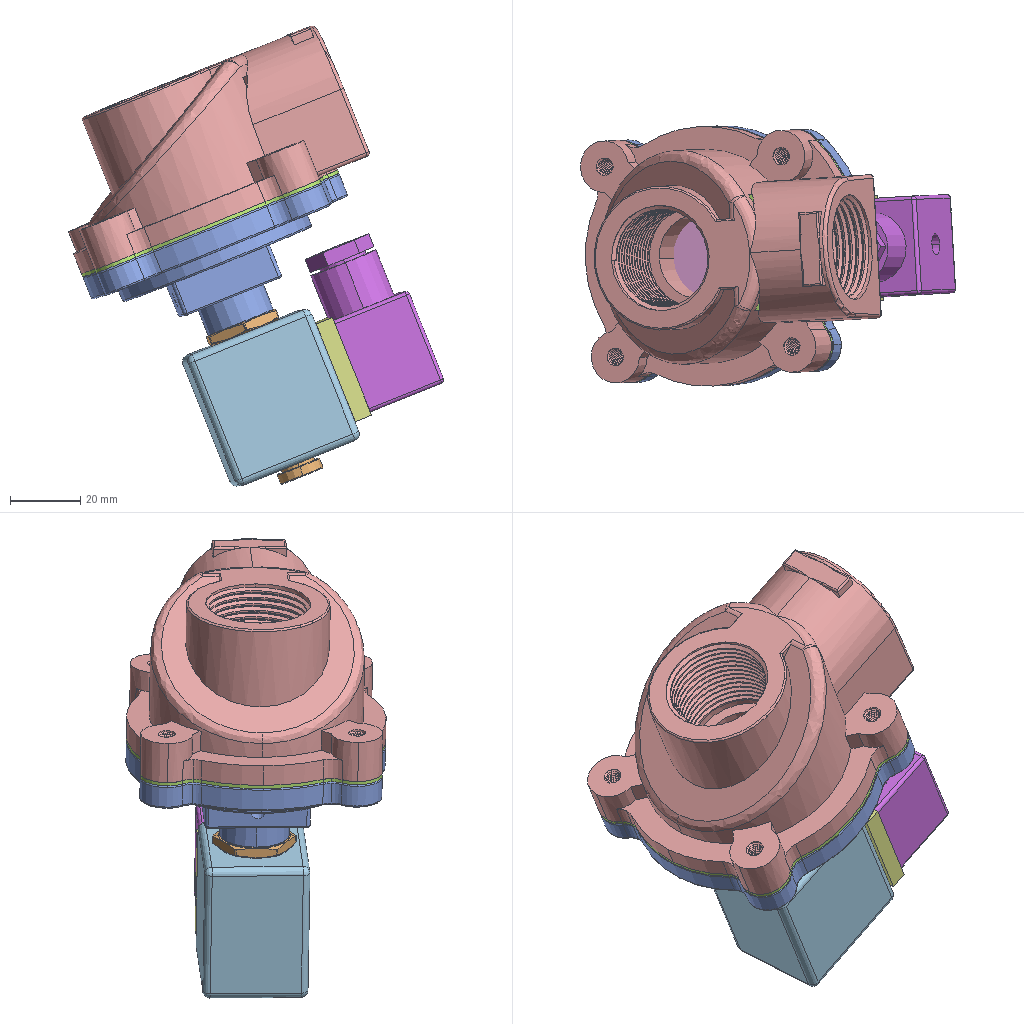Assembly | SolidWorks | 12 different items | 12 placed | box 107 x 74 x 131 mm
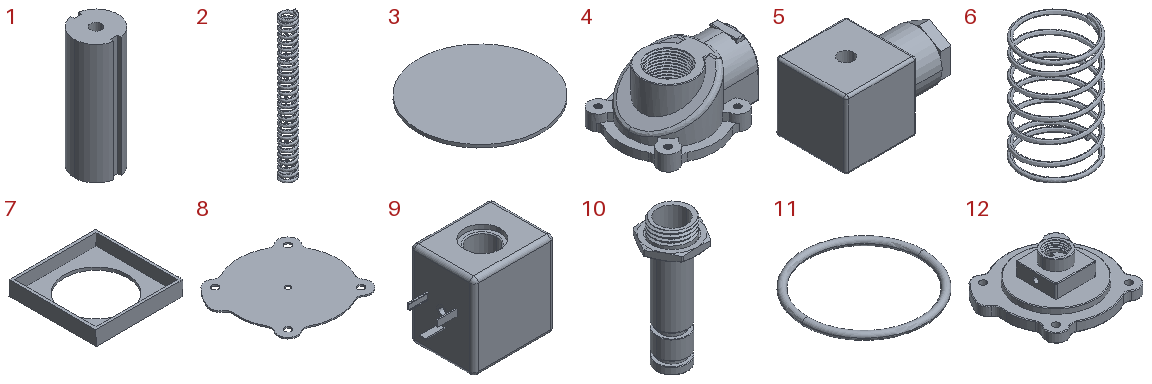Parts list (item | quantity | size | volume | features):
1 | x1 | 12 x 11.832 x 33 mm | 3415 mm3 | features ICE 5, Extrusion 1, MirrorPattern 1
2 | x1 | 3 x 3 x 28.006 mm | 41.608 mm3 | features Helix 1, Sweep 1
3 | x1 | 40 x 40 x 3 mm | 1760 mm3 | features ICE 2, Extrusion 1
4 | x1 | 88 x 74 x 41.7 mm | 68269 mm3 | features ICE 16, Fillet 11, CirPattern 3, SweepThread 3, Chamfer 1, Extrusion 1, Helix 1
5 | x1 | 47 x 28 x 27 mm | 22698 mm3 | features ICE 4, Cut 3, BossThin 1, Extrusion 1, Fillet 1
6 | x1 | 17 x 17 x 27.04 mm | 272.389 mm3 | features Helix 1, Sweep 1
7 | x1 | 30 x 30 x 5 mm | 983.867 mm3 | features BossThin 1, Extrusion 1, ICE 1
8 | x1 | 79.627 x 74 x 1 mm | 4806 mm3 | features Cut 1, Extrusion 1
9 | x1 | 47 x 30 x 40 mm | 39521 mm3 | features ICE 7, Fillet 2, Extrusion 1, MirrorPattern 1
10 | x1 | 23.845 x 20.785 x 53 mm | 4184 mm3 | features Cut 4, Fillet 4, ICE 2, Chamfer 1, Extrusion 1, RefAxis 1, RevCut 1, SweepThread 1
11 | x1 | 17.5 x 17.5 x 1 mm | 40.712 mm3 | features Sweep 1
12 | x1 | 79.627 x 74 x 30 mm | 34893 mm3 | features Fillet 12, ICE 11, Cut 9, HoleWzd 2, MirrorPattern 2, CirPattern 1, Extrusion 1, SweepThread 1
Mates (type | each side: item.copy, entity, surface, feature):
Concentric | 4.1 face cylinder CirPattern1 | 12.1 face cylinder Boss-Extrude1 | 2 times
Concentric | 4.1 face cylinder CirPattern1 | 8.1 face cylinder Boss-Extrude1 | 2 times
InPlace | 8.1 face plane Boss-Extrude1 | 3.1 plane
InPlace | assembly face | assembly plane
Concentric | assembly face | 11.1 select_type:24
Tangent | assembly face | 11.1 face torus Sweep1
Concentric | 12.1 face cylinder Boss-Extrude8 | 10.1 face cylinder Boss-Extrude2
Concentric | 11.1 select_type:24 | 10.1 face cylinder Boss-Extrude2
Tangent | 11.1 face torus Sweep1 | 10.1 face plane Cut-Extrude4
Coincident | 11.1 select_type:24 | 6.1 select_type:24
Lock | 3.1 select_type:0 | 6.1 select_type:0
Coincident | 4.1 face plane Boss-Extrude1 | 8.1 face plane Boss-Extrude1
Coincident | 12.1 face plane Boss-Extrude1 | 8.1 face plane Boss-Extrude1
Coincident | 11.1 select_type:24 | 2.1 select_type:24
Concentric | 12.1 face cylinder Boss-Extrude8 | 1.1 face cylinder Boss-Extrude1
Coincident | 12.1 face plane Cut-Extrude7 | 1.1 face plane Boss-Extrude1
Coincident | 12.1 face plane Boss-Extrude8 | 10.1 face plane Boss-Extrude3
Parallel | 4.1 face plane Boss-Extrude4 | 10.1 face plane Boss-Extrude3
Concentric | 10.1 face cylinder Boss-Extrude2 | 9.1 face cylinder Cut-Extrude1
Coincident | 10.1 face plane Boss-Extrude3 | 9.1 face plane Boss-Extrude1
InPlace | 9.1 face plane Boss-Extrude2 | assembly plane
Coincident | 7.1 face plane Extrude-Thin1 | 5.1 face plane Boss-Extrude1 | 2 times
Coincident | 9.1 face plane Boss-Extrude1 | 7.1 face plane Boss-Extrude1
Concentric | 9.1 face cylinder Cut-Extrude4 | 5.1 face cylinder Cut-Extrude1
Coincident | 7.1 face plane Boss-Extrude1 | 5.1 face plane Boss-Extrude1
Lock | 2.1 select_type:0 | 1.1 select_type:0